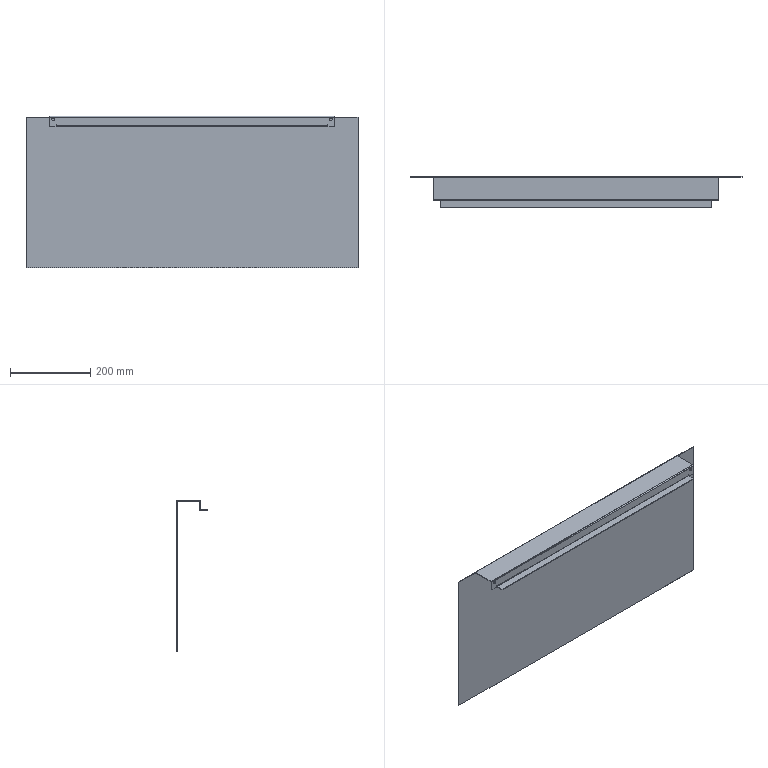Part | STEP file | Electrical Cabinet 2 | 1 solid | 40 faces | box 828 x 78 x 378 mm | volume 762303 mm3 | plane 24 | cylinder 16 | commonest cylinder face diameters 1 x9 7 x4 5 x3
STEP:
#1=CARTESIAN_POINT('',(684.62,-58.,322.807));
#2=VERTEX_POINT('',#1);
#3=CARTESIAN_POINT('',(684.62,-58.,329.807));
#4=VERTEX_POINT('',#3);
#5=CARTESIAN_POINT('',(684.62,-58.,326.307));
#6=DIRECTION('',(0.,1.,0.));
#7=DIRECTION('',(0.,0.,-1.));
#8=AXIS2_PLACEMENT_3D('',#5,#6,#7);
#9=CIRCLE('',#8,3.5);
#10=EDGE_CURVE('',#2,#4,#9,.T.);
#11=ORIENTED_EDGE('',*,*,#10,.T.);
#12=CARTESIAN_POINT('',(684.62,-60.,329.807));
#13=VERTEX_POINT('',#12);
#14=CARTESIAN_POINT('',(684.62,-50.,329.807));
#15=DIRECTION('',(0.,-1.,0.));
#16=VECTOR('',#15,1000.);
#17=LINE('',#14,#16);
#18=EDGE_CURVE('',#4,#13,#17,.T.);
#19=ORIENTED_EDGE('',*,*,#18,.T.);
#20=CARTESIAN_POINT('',(684.62,-60.,322.807));
#21=VERTEX_POINT('',#20);
#22=CARTESIAN_POINT('',(684.62,-60.,326.307));
#23=DIRECTION('',(0.,1.,0.));
#24=DIRECTION('',(0.,0.,-1.));
#25=AXIS2_PLACEMENT_3D('',#22,#23,#24);
#26=CIRCLE('',#25,3.5);
#27=EDGE_CURVE('',#21,#13,#26,.T.);
#28=ORIENTED_EDGE('',*,*,#27,.F.);
#29=CARTESIAN_POINT('',(684.62,-50.,322.807));
#30=DIRECTION('',(0.,-1.,0.));
#31=VECTOR('',#30,1000.);
#32=LINE('',#29,#31);
#33=EDGE_CURVE('',#2,#21,#32,.T.);
#34=ORIENTED_EDGE('',*,*,#33,.F.);
#35=EDGE_LOOP('',(#11,#19,#28,#34));
#36=FACE_OUTER_BOUND('',#35,.T.);
#37=CARTESIAN_POINT('',(684.62,-50.,326.307));
#38=DIRECTION('',(0.,-1.,0.));
#39=DIRECTION('',(0.,0.,-1.));
#40=AXIS2_PLACEMENT_3D('',#37,#38,#39);
#41=CYLINDRICAL_SURFACE('',#40,3.5);
#42=ADVANCED_FACE('',(#36),#41,.F.);
#43=CARTESIAN_POINT('',(-7.38,-58.,322.807));
#44=VERTEX_POINT('',#43);
#45=CARTESIAN_POINT('',(-7.38,-58.,329.807));
#46=VERTEX_POINT('',#45);
#47=CARTESIAN_POINT('',(-7.38,-58.,326.307));
#48=DIRECTION('',(0.,1.,0.));
#49=DIRECTION('',(0.,0.,-1.));
#50=AXIS2_PLACEMENT_3D('',#47,#48,#49);
#51=CIRCLE('',#50,3.5);
#52=EDGE_CURVE('',#44,#46,#51,.T.);
#53=ORIENTED_EDGE('',*,*,#52,.T.);
#54=CARTESIAN_POINT('',(-7.38,-60.,329.807));
#55=VERTEX_POINT('',#54);
#56=CARTESIAN_POINT('',(-7.38,-50.,329.807));
#57=DIRECTION('',(0.,-1.,0.));
#58=VECTOR('',#57,1000.);
#59=LINE('',#56,#58);
#60=EDGE_CURVE('',#46,#55,#59,.T.);
#61=ORIENTED_EDGE('',*,*,#60,.T.);
#62=CARTESIAN_POINT('',(-7.38,-60.,322.807));
#63=VERTEX_POINT('',#62);
#64=CARTESIAN_POINT('',(-7.38,-60.,326.307));
#65=DIRECTION('',(0.,1.,0.));
#66=DIRECTION('',(0.,0.,-1.));
#67=AXIS2_PLACEMENT_3D('',#64,#65,#66);
#68=CIRCLE('',#67,3.5);
#69=EDGE_CURVE('',#63,#55,#68,.T.);
#70=ORIENTED_EDGE('',*,*,#69,.F.);
#71=CARTESIAN_POINT('',(-7.38,-50.,322.807));
#72=DIRECTION('',(0.,-1.,0.));
#73=VECTOR('',#72,1000.);
#74=LINE('',#71,#73);
#75=EDGE_CURVE('',#44,#63,#74,.T.);
#76=ORIENTED_EDGE('',*,*,#75,.F.);
#77=EDGE_LOOP('',(#53,#61,#70,#76));
#78=FACE_OUTER_BOUND('',#77,.T.);
#79=CARTESIAN_POINT('',(-7.38,-50.,326.307));
#80=DIRECTION('',(0.,-1.,0.));
#81=DIRECTION('',(0.,0.,-1.));
#82=AXIS2_PLACEMENT_3D('',#79,#80,#81);
#83=CYLINDRICAL_SURFACE('',#82,3.5);
#84=ADVANCED_FACE('',(#78),#83,.F.);
#85=CARTESIAN_POINT('',(677.12,-60.,313.307));
#86=VERTEX_POINT('',#85);
#87=CARTESIAN_POINT('',(677.62,-60.,312.807));
#88=VERTEX_POINT('',#87);
#89=CARTESIAN_POINT('',(677.12,-60.,312.807));
#90=DIRECTION('',(0.,1.,0.));
#91=DIRECTION('',(0.,0.,1.));
#92=AXIS2_PLACEMENT_3D('',#89,#90,#91);
#93=CIRCLE('',#92,0.5);
#94=EDGE_CURVE('',#86,#88,#93,.T.);
#95=ORIENTED_EDGE('',*,*,#94,.F.);
#96=CARTESIAN_POINT('',(677.12,-58.,313.307));
#97=VERTEX_POINT('',#96);
#98=CARTESIAN_POINT('',(677.12,-60.,313.307));
#99=DIRECTION('',(0.,1.,0.));
#100=VECTOR('',#99,1000.);
#101=LINE('',#98,#100);
#102=EDGE_CURVE('',#86,#97,#101,.T.);
#103=ORIENTED_EDGE('',*,*,#102,.T.);
#104=CARTESIAN_POINT('',(677.62,-58.,312.807));
#105=VERTEX_POINT('',#104);
#106=CARTESIAN_POINT('',(677.12,-58.,312.807));
#107=DIRECTION('',(0.,-1.,0.));
#108=DIRECTION('',(0.,0.,1.));
#109=AXIS2_PLACEMENT_3D('',#106,#107,#108);
#110=CIRCLE('',#109,0.5);
#111=EDGE_CURVE('',#105,#97,#110,.T.);
#112=ORIENTED_EDGE('',*,*,#111,.F.);
#113=CARTESIAN_POINT('',(677.62,-60.,312.807));
#114=DIRECTION('',(0.,1.,0.));
#115=VECTOR('',#114,1000.);
#116=LINE('',#113,#115);
#117=EDGE_CURVE('',#88,#105,#116,.T.);
#118=ORIENTED_EDGE('',*,*,#117,.F.);
#119=EDGE_LOOP('',(#95,#103,#112,#118));
#120=FACE_OUTER_BOUND('',#119,.T.);
#121=CARTESIAN_POINT('',(677.12,-60.,312.807));
#122=DIRECTION('',(0.,1.,0.));
#123=DIRECTION('',(0.,0.,1.));
#124=AXIS2_PLACEMENT_3D('',#121,#122,#123);
#125=CYLINDRICAL_SURFACE('',#124,0.5);
#126=ADVANCED_FACE('',(#120),#125,.F.);
#127=CARTESIAN_POINT('',(0.1199,-60.,313.307));
#128=VERTEX_POINT('',#127);
#129=CARTESIAN_POINT('',(0.6199,-60.,312.807));
#130=VERTEX_POINT('',#129);
#131=CARTESIAN_POINT('',(0.1199,-60.,312.807));
#132=DIRECTION('',(0.,1.,0.));
#133=DIRECTION('',(0.,0.,1.));
#134=AXIS2_PLACEMENT_3D('',#131,#132,#133);
#135=CIRCLE('',#134,0.5);
#136=EDGE_CURVE('',#128,#130,#135,.T.);
#137=ORIENTED_EDGE('',*,*,#136,.F.);
#138=CARTESIAN_POINT('',(0.1199,-58.,313.307));
#139=VERTEX_POINT('',#138);
#140=CARTESIAN_POINT('',(0.1199,-60.,313.307));
#141=DIRECTION('',(0.,1.,0.));
#142=VECTOR('',#141,1000.);
#143=LINE('',#140,#142);
#144=EDGE_CURVE('',#128,#139,#143,.T.);
#145=ORIENTED_EDGE('',*,*,#144,.T.);
#146=CARTESIAN_POINT('',(0.6199,-58.,312.807));
#147=VERTEX_POINT('',#146);
#148=CARTESIAN_POINT('',(0.1199,-58.,312.807));
#149=DIRECTION('',(0.,-1.,0.));
#150=DIRECTION('',(0.,0.,1.));
#151=AXIS2_PLACEMENT_3D('',#148,#149,#150);
#152=CIRCLE('',#151,0.5);
#153=EDGE_CURVE('',#147,#139,#152,.T.);
#154=ORIENTED_EDGE('',*,*,#153,.F.);
#155=CARTESIAN_POINT('',(0.6199,-60.,312.807));
#156=DIRECTION('',(0.,1.,0.));
#157=VECTOR('',#156,1000.);
#158=LINE('',#155,#157);
#159=EDGE_CURVE('',#130,#147,#158,.T.);
#160=ORIENTED_EDGE('',*,*,#159,.F.);
#161=EDGE_LOOP('',(#137,#145,#154,#160));
#162=FACE_OUTER_BOUND('',#161,.T.);
#163=CARTESIAN_POINT('',(0.1199,-60.,312.807));
#164=DIRECTION('',(0.,1.,0.));
#165=DIRECTION('',(0.,0.,1.));
#166=AXIS2_PLACEMENT_3D('',#163,#164,#165);
#167=CYLINDRICAL_SURFACE('',#166,0.5);
#168=ADVANCED_FACE('',(#162),#167,.F.);
#169=CARTESIAN_POINT('',(695.62,-2.,332.307));
#170=VERTEX_POINT('',#169);
#171=CARTESIAN_POINT('',(752.62,-2.,332.307));
#172=VERTEX_POINT('',#171);
#173=CARTESIAN_POINT('',(0.,-2.,332.307));
#174=DIRECTION('',(1.,0.,0.));
#175=VECTOR('',#174,1000.);
#176=LINE('',#173,#175);
#177=EDGE_CURVE('',#170,#172,#176,.T.);
#178=ORIENTED_EDGE('',*,*,#177,.F.);
#179=CARTESIAN_POINT('',(695.62,-2.,330.807));
#180=VERTEX_POINT('',#179);
#181=CARTESIAN_POINT('',(695.62,-2.,330.807));
#182=DIRECTION('',(0.,0.,1.));
#183=VECTOR('',#182,1000.);
#184=LINE('',#181,#183);
#185=EDGE_CURVE('',#180,#170,#184,.T.);
#186=ORIENTED_EDGE('',*,*,#185,.F.);
#187=CARTESIAN_POINT('',(694.62,-2.,330.807));
#188=VERTEX_POINT('',#187);
#189=CARTESIAN_POINT('',(695.12,-2.,330.807));
#190=DIRECTION('',(0.,1.,0.));
#191=DIRECTION('',(0.,0.,1.));
#192=AXIS2_PLACEMENT_3D('',#189,#190,#191);
#193=CIRCLE('',#192,0.5);
#194=EDGE_CURVE('',#180,#188,#193,.T.);
#195=ORIENTED_EDGE('',*,*,#194,.T.);
#196=CARTESIAN_POINT('',(694.62,-2.,331.807));
#197=VERTEX_POINT('',#196);
#198=CARTESIAN_POINT('',(694.62,-2.,331.807));
#199=DIRECTION('',(0.,0.,-1.));
#200=VECTOR('',#199,1000.);
#201=LINE('',#198,#200);
#202=EDGE_CURVE('',#197,#188,#201,.T.);
#203=ORIENTED_EDGE('',*,*,#202,.F.);
#204=CARTESIAN_POINT('',(-17.38,-2.,331.807));
#205=VERTEX_POINT('',#204);
#206=CARTESIAN_POINT('',(0.,-2.,331.807));
#207=DIRECTION('',(1.,0.,0.));
#208=VECTOR('',#207,1000.);
#209=LINE('',#206,#208);
#210=EDGE_CURVE('',#205,#197,#209,.T.);
#211=ORIENTED_EDGE('',*,*,#210,.F.);
#212=CARTESIAN_POINT('',(-17.38,-2.,330.807));
#213=VERTEX_POINT('',#212);
#214=CARTESIAN_POINT('',(-17.38,-2.,330.807));
#215=DIRECTION('',(0.,0.,1.));
#216=VECTOR('',#215,1000.);
#217=LINE('',#214,#216);
#218=EDGE_CURVE('',#213,#205,#217,.T.);
#219=ORIENTED_EDGE('',*,*,#218,.F.);
#220=CARTESIAN_POINT('',(-18.38,-2.,330.807));
#221=VERTEX_POINT('',#220);
#222=CARTESIAN_POINT('',(-17.88,-2.,330.807));
#223=DIRECTION('',(0.,1.,0.));
#224=DIRECTION('',(0.,0.,1.));
#225=AXIS2_PLACEMENT_3D('',#222,#223,#224);
#226=CIRCLE('',#225,0.5);
#227=EDGE_CURVE('',#213,#221,#226,.T.);
#228=ORIENTED_EDGE('',*,*,#227,.T.);
#229=CARTESIAN_POINT('',(-18.38,-2.,332.307));
#230=VERTEX_POINT('',#229);
#231=CARTESIAN_POINT('',(-18.38,-2.,334.307));
#232=DIRECTION('',(0.,0.,-1.));
#233=VECTOR('',#232,1000.);
#234=LINE('',#231,#233);
#235=EDGE_CURVE('',#230,#221,#234,.T.);
#236=ORIENTED_EDGE('',*,*,#235,.F.);
#237=CARTESIAN_POINT('',(-75.38,-2.,332.307));
#238=VERTEX_POINT('',#237);
#239=CARTESIAN_POINT('',(0.,-2.,332.307));
#240=DIRECTION('',(1.,0.,0.));
#241=VECTOR('',#240,1000.);
#242=LINE('',#239,#241);
#243=EDGE_CURVE('',#238,#230,#242,.T.);
#244=ORIENTED_EDGE('',*,*,#243,.F.);
#245=CARTESIAN_POINT('',(-75.38,-2.,-43.693));
#246=VERTEX_POINT('',#245);
#247=CARTESIAN_POINT('',(-75.38,-2.,0.));
#248=DIRECTION('',(0.,0.,1.));
#249=VECTOR('',#248,1000.);
#250=LINE('',#247,#249);
#251=EDGE_CURVE('',#246,#238,#250,.T.);
#252=ORIENTED_EDGE('',*,*,#251,.F.);
#253=CARTESIAN_POINT('',(752.62,-2.,-43.693));
#254=VERTEX_POINT('',#253);
#255=CARTESIAN_POINT('',(0.,-2.,-43.693));
#256=DIRECTION('',(-1.,0.,0.));
#257=VECTOR('',#256,1000.);
#258=LINE('',#255,#257);
#259=EDGE_CURVE('',#254,#246,#258,.T.);
#260=ORIENTED_EDGE('',*,*,#259,.F.);
#261=CARTESIAN_POINT('',(752.62,-2.,0.));
#262=DIRECTION('',(0.,0.,-1.));
#263=VECTOR('',#262,1000.);
#264=LINE('',#261,#263);
#265=EDGE_CURVE('',#172,#254,#264,.T.);
#266=ORIENTED_EDGE('',*,*,#265,.F.);
#267=EDGE_LOOP('',(#178,#186,#195,#203,#211,#219,#228,#236,#244,#252,#260,#266));
#268=FACE_OUTER_BOUND('',#267,.T.);
#269=CARTESIAN_POINT('',(0.,-2.,0.));
#270=DIRECTION('',(0.,1.,0.));
#271=DIRECTION('',(0.,0.,1.));
#272=AXIS2_PLACEMENT_3D('',#269,#270,#271);
#273=PLANE('',#272);
#274=ADVANCED_FACE('',(#268),#273,.F.);
#275=CARTESIAN_POINT('',(752.62,0.,-43.693));
#276=VERTEX_POINT('',#275);
#277=CARTESIAN_POINT('',(752.62,-2.,-43.693));
#278=DIRECTION('',(0.,1.,0.));
#279=VECTOR('',#278,1000.);
#280=LINE('',#277,#279);
#281=EDGE_CURVE('',#254,#276,#280,.T.);
#282=ORIENTED_EDGE('',*,*,#281,.T.);
#283=CARTESIAN_POINT('',(752.62,0.,332.307));
#284=VERTEX_POINT('',#283);
#285=CARTESIAN_POINT('',(752.62,0.,-43.693));
#286=DIRECTION('',(0.,0.,1.));
#287=VECTOR('',#286,1000.);
#288=LINE('',#285,#287);
#289=EDGE_CURVE('',#276,#284,#288,.T.);
#290=ORIENTED_EDGE('',*,*,#289,.T.);
#291=CARTESIAN_POINT('',(752.62,-2.,332.307));
#292=DIRECTION('',(0.,-1.,0.));
#293=VECTOR('',#292,1000.);
#294=LINE('',#291,#293);
#295=EDGE_CURVE('',#284,#172,#294,.T.);
#296=ORIENTED_EDGE('',*,*,#295,.T.);
#297=ORIENTED_EDGE('',*,*,#265,.T.);
#298=EDGE_LOOP('',(#282,#290,#296,#297));
#299=FACE_OUTER_BOUND('',#298,.T.);
#300=CARTESIAN_POINT('',(752.62,-2.,-43.693));
#301=DIRECTION('',(1.,0.,0.));
#302=DIRECTION('',(0.,0.,-1.));
#303=AXIS2_PLACEMENT_3D('',#300,#301,#302);
#304=PLANE('',#303);
#305=ADVANCED_FACE('',(#299),#304,.T.);
#306=CARTESIAN_POINT('',(695.62,0.,332.307));
#307=VERTEX_POINT('',#306);
#308=CARTESIAN_POINT('',(695.62,0.,332.307));
#309=DIRECTION('',(1.,0.,0.));
#310=VECTOR('',#309,1000.);
#311=LINE('',#308,#310);
#312=EDGE_CURVE('',#307,#284,#311,.T.);
#313=ORIENTED_EDGE('',*,*,#312,.F.);
#314=CARTESIAN_POINT('',(695.62,-10.,332.307));
#315=DIRECTION('',(0.,1.,0.));
#316=VECTOR('',#315,1000.);
#317=LINE('',#314,#316);
#318=EDGE_CURVE('',#170,#307,#317,.T.);
#319=ORIENTED_EDGE('',*,*,#318,.F.);
#320=ORIENTED_EDGE('',*,*,#177,.T.);
#321=ORIENTED_EDGE('',*,*,#295,.F.);
#322=EDGE_LOOP('',(#313,#319,#320,#321));
#323=FACE_OUTER_BOUND('',#322,.T.);
#324=CARTESIAN_POINT('',(695.62,-10.,332.307));
#325=DIRECTION('',(0.,0.,-1.));
#326=DIRECTION('',(-1.,0.,0.));
#327=AXIS2_PLACEMENT_3D('',#324,#325,#326);
#328=PLANE('',#327);
#329=ADVANCED_FACE('',(#323),#328,.F.);
#330=CARTESIAN_POINT('',(694.62,-2.5,332.307));
#331=VERTEX_POINT('',#330);
#332=CARTESIAN_POINT('',(694.62,-2.5,331.807));
#333=DIRECTION('',(-1.,0.,0.));
#334=DIRECTION('',(0.,0.,1.));
#335=AXIS2_PLACEMENT_3D('',#332,#333,#334);
#336=CIRCLE('',#335,0.5);
#337=EDGE_CURVE('',#331,#197,#336,.T.);
#338=ORIENTED_EDGE('',*,*,#337,.F.);
#339=CARTESIAN_POINT('',(-17.38,-2.5,332.307));
#340=VERTEX_POINT('',#339);
#341=CARTESIAN_POINT('',(-17.38,-2.5,332.307));
#342=DIRECTION('',(1.,0.,0.));
#343=VECTOR('',#342,1000.);
#344=LINE('',#341,#343);
#345=EDGE_CURVE('',#340,#331,#344,.T.);
#346=ORIENTED_EDGE('',*,*,#345,.F.);
#347=CARTESIAN_POINT('',(-17.38,-2.5,331.807));
#348=DIRECTION('',(-1.,0.,0.));
#349=DIRECTION('',(0.,0.,1.));
#350=AXIS2_PLACEMENT_3D('',#347,#348,#349);
#351=CIRCLE('',#350,0.5);
#352=EDGE_CURVE('',#340,#205,#351,.T.);
#353=ORIENTED_EDGE('',*,*,#352,.T.);
#354=ORIENTED_EDGE('',*,*,#210,.T.);
#355=EDGE_LOOP('',(#338,#346,#353,#354));
#356=FACE_OUTER_BOUND('',#355,.T.);
#357=CARTESIAN_POINT('',(-17.38,-2.5,331.807));
#358=DIRECTION('',(-1.,0.,0.));
#359=DIRECTION('',(0.,0.,1.));
#360=AXIS2_PLACEMENT_3D('',#357,#358,#359);
#361=CYLINDRICAL_SURFACE('',#360,0.5);
#362=ADVANCED_FACE('',(#356),#361,.F.);
#363=CARTESIAN_POINT('',(-75.38,0.,332.307));
#364=VERTEX_POINT('',#363);
#365=CARTESIAN_POINT('',(-18.38,0.,332.307));
#366=VERTEX_POINT('',#365);
#367=CARTESIAN_POINT('',(-75.38,0.,332.307));
#368=DIRECTION('',(1.,0.,0.));
#369=VECTOR('',#368,1000.);
#370=LINE('',#367,#369);
#371=EDGE_CURVE('',#364,#366,#370,.T.);
#372=ORIENTED_EDGE('',*,*,#371,.F.);
#373=CARTESIAN_POINT('',(-75.38,-10.,332.307));
#374=DIRECTION('',(0.,1.,0.));
#375=VECTOR('',#374,1000.);
#376=LINE('',#373,#375);
#377=EDGE_CURVE('',#238,#364,#376,.T.);
#378=ORIENTED_EDGE('',*,*,#377,.F.);
#379=ORIENTED_EDGE('',*,*,#243,.T.);
#380=CARTESIAN_POINT('',(-18.38,-10.,332.307));
#381=DIRECTION('',(0.,-1.,0.));
#382=VECTOR('',#381,1000.);
#383=LINE('',#380,#382);
#384=EDGE_CURVE('',#366,#230,#383,.T.);
#385=ORIENTED_EDGE('',*,*,#384,.F.);
#386=EDGE_LOOP('',(#372,#378,#379,#385));
#387=FACE_OUTER_BOUND('',#386,.T.);
#388=CARTESIAN_POINT('',(-75.38,-10.,332.307));
#389=DIRECTION('',(0.,0.,-1.));
#390=DIRECTION('',(-1.,0.,0.));
#391=AXIS2_PLACEMENT_3D('',#388,#389,#390);
#392=PLANE('',#391);
#393=ADVANCED_FACE('',(#387),#392,.F.);
#394=CARTESIAN_POINT('',(-75.38,0.,-43.693));
#395=VERTEX_POINT('',#394);
#396=CARTESIAN_POINT('',(-75.38,-2.,-43.693));
#397=DIRECTION('',(0.,-1.,0.));
#398=VECTOR('',#397,1000.);
#399=LINE('',#396,#398);
#400=EDGE_CURVE('',#395,#246,#399,.T.);
#401=ORIENTED_EDGE('',*,*,#400,.T.);
#402=ORIENTED_EDGE('',*,*,#251,.T.);
#403=ORIENTED_EDGE('',*,*,#377,.T.);
#404=CARTESIAN_POINT('',(-75.38,0.,-43.693));
#405=DIRECTION('',(0.,0.,-1.));
#406=VECTOR('',#405,1000.);
#407=LINE('',#404,#406);
#408=EDGE_CURVE('',#364,#395,#407,.T.);
#409=ORIENTED_EDGE('',*,*,#408,.T.);
#410=EDGE_LOOP('',(#401,#402,#403,#409));
#411=FACE_OUTER_BOUND('',#410,.T.);
#412=CARTESIAN_POINT('',(-75.38,-2.,-43.693));
#413=DIRECTION('',(-1.,0.,0.));
#414=DIRECTION('',(0.,0.,1.));
#415=AXIS2_PLACEMENT_3D('',#412,#413,#414);
#416=PLANE('',#415);
#417=ADVANCED_FACE('',(#411),#416,.T.);
#418=ORIENTED_EDGE('',*,*,#259,.T.);
#419=ORIENTED_EDGE('',*,*,#400,.F.);
#420=CARTESIAN_POINT('',(-75.38,0.,-43.693));
#421=DIRECTION('',(1.,0.,0.));
#422=VECTOR('',#421,1000.);
#423=LINE('',#420,#422);
#424=EDGE_CURVE('',#395,#276,#423,.T.);
#425=ORIENTED_EDGE('',*,*,#424,.T.);
#426=ORIENTED_EDGE('',*,*,#281,.F.);
#427=EDGE_LOOP('',(#418,#419,#425,#426));
#428=FACE_OUTER_BOUND('',#427,.T.);
#429=CARTESIAN_POINT('',(-75.38,-2.,-43.693));
#430=DIRECTION('',(0.,0.,-1.));
#431=DIRECTION('',(-1.,0.,0.));
#432=AXIS2_PLACEMENT_3D('',#429,#430,#431);
#433=PLANE('',#432);
#434=ADVANCED_FACE('',(#428),#433,.T.);
#435=CARTESIAN_POINT('',(694.62,0.,330.807));
#436=VERTEX_POINT('',#435);
#437=CARTESIAN_POINT('',(695.62,0.,330.807));
#438=VERTEX_POINT('',#437);
#439=CARTESIAN_POINT('',(695.12,0.,330.807));
#440=DIRECTION('',(0.,-1.,0.));
#441=DIRECTION('',(0.,0.,1.));
#442=AXIS2_PLACEMENT_3D('',#439,#440,#441);
#443=CIRCLE('',#442,0.5);
#444=EDGE_CURVE('',#436,#438,#443,.T.);
#445=ORIENTED_EDGE('',*,*,#444,.T.);
#446=CARTESIAN_POINT('',(695.62,0.,0.));
#447=DIRECTION('',(0.,0.,1.));
#448=VECTOR('',#447,1000.);
#449=LINE('',#446,#448);
#450=EDGE_CURVE('',#438,#307,#449,.T.);
#451=ORIENTED_EDGE('',*,*,#450,.T.);
#452=ORIENTED_EDGE('',*,*,#312,.T.);
#453=ORIENTED_EDGE('',*,*,#289,.F.);
#454=ORIENTED_EDGE('',*,*,#424,.F.);
#455=ORIENTED_EDGE('',*,*,#408,.F.);
#456=ORIENTED_EDGE('',*,*,#371,.T.);
#457=CARTESIAN_POINT('',(-18.38,0.,330.807));
#458=VERTEX_POINT('',#457);
#459=CARTESIAN_POINT('',(-18.38,0.,0.));
#460=DIRECTION('',(0.,0.,-1.));
#461=VECTOR('',#460,1000.);
#462=LINE('',#459,#461);
#463=EDGE_CURVE('',#366,#458,#462,.T.);
#464=ORIENTED_EDGE('',*,*,#463,.T.);
#465=CARTESIAN_POINT('',(-17.38,0.,330.807));
#466=VERTEX_POINT('',#465);
#467=CARTESIAN_POINT('',(-17.88,0.,330.807));
#468=DIRECTION('',(0.,-1.,0.));
#469=DIRECTION('',(0.,0.,1.));
#470=AXIS2_PLACEMENT_3D('',#467,#468,#469);
#471=CIRCLE('',#470,0.5);
#472=EDGE_CURVE('',#458,#466,#471,.T.);
#473=ORIENTED_EDGE('',*,*,#472,.T.);
#474=CARTESIAN_POINT('',(-17.38,0.,331.807));
#475=VERTEX_POINT('',#474);
#476=CARTESIAN_POINT('',(-17.38,0.,330.807));
#477=DIRECTION('',(0.,0.,-1.));
#478=VECTOR('',#477,1000.);
#479=LINE('',#476,#478);
#480=EDGE_CURVE('',#475,#466,#479,.T.);
#481=ORIENTED_EDGE('',*,*,#480,.F.);
#482=CARTESIAN_POINT('',(694.62,0.,331.807));
#483=VERTEX_POINT('',#482);
#484=CARTESIAN_POINT('',(0.,0.,331.807));
#485=DIRECTION('',(1.,0.,0.));
#486=VECTOR('',#485,1000.);
#487=LINE('',#484,#486);
#488=EDGE_CURVE('',#475,#483,#487,.T.);
#489=ORIENTED_EDGE('',*,*,#488,.T.);
#490=CARTESIAN_POINT('',(694.62,0.,331.807));
#491=DIRECTION('',(0.,0.,1.));
#492=VECTOR('',#491,1000.);
#493=LINE('',#490,#492);
#494=EDGE_CURVE('',#436,#483,#493,.T.);
#495=ORIENTED_EDGE('',*,*,#494,.F.);
#496=EDGE_LOOP('',(#445,#451,#452,#453,#454,#455,#456,#464,#473,#481,#489,#495));
#497=FACE_OUTER_BOUND('',#496,.T.);
#498=CARTESIAN_POINT('',(0.,0.,0.));
#499=DIRECTION('',(0.,1.,0.));
#500=DIRECTION('',(0.,0.,1.));
#501=AXIS2_PLACEMENT_3D('',#498,#499,#500);
#502=PLANE('',#501);
#503=ADVANCED_FACE('',(#497),#502,.T.);
#504=CARTESIAN_POINT('',(695.62,-2.,330.807));
#505=DIRECTION('',(0.,-1.,0.));
#506=VECTOR('',#505,1000.);
#507=LINE('',#504,#506);
#508=EDGE_CURVE('',#438,#180,#507,.T.);
#509=ORIENTED_EDGE('',*,*,#508,.T.);
#510=ORIENTED_EDGE('',*,*,#185,.T.);
#511=ORIENTED_EDGE('',*,*,#318,.T.);
#512=ORIENTED_EDGE('',*,*,#450,.F.);
#513=EDGE_LOOP('',(#509,#510,#511,#512));
#514=FACE_OUTER_BOUND('',#513,.T.);
#515=CARTESIAN_POINT('',(695.62,-2.,330.807));
#516=DIRECTION('',(-1.,0.,0.));
#517=DIRECTION('',(0.,0.,1.));
#518=AXIS2_PLACEMENT_3D('',#515,#516,#517);
#519=PLANE('',#518);
#520=ADVANCED_FACE('',(#514),#519,.T.);
#521=CARTESIAN_POINT('',(-17.38,-57.5,332.307));
#522=VERTEX_POINT('',#521);
#523=CARTESIAN_POINT('',(-17.38,0.,332.307));
#524=DIRECTION('',(0.,-1.,0.));
#525=VECTOR('',#524,1000.);
#526=LINE('',#523,#525);
#527=EDGE_CURVE('',#340,#522,#526,.T.);
#528=ORIENTED_EDGE('',*,*,#527,.F.);
#529=ORIENTED_EDGE('',*,*,#345,.T.);
#530=CARTESIAN_POINT('',(694.62,-57.5,332.307));
#531=VERTEX_POINT('',#530);
#532=CARTESIAN_POINT('',(694.62,0.,332.307));
#533=DIRECTION('',(0.,1.,0.));
#534=VECTOR('',#533,1000.);
#535=LINE('',#532,#534);
#536=EDGE_CURVE('',#531,#331,#535,.T.);
#537=ORIENTED_EDGE('',*,*,#536,.F.);
#538=CARTESIAN_POINT('',(0.,-57.5,332.307));
#539=DIRECTION('',(1.,0.,0.));
#540=VECTOR('',#539,1000.);
#541=LINE('',#538,#540);
#542=EDGE_CURVE('',#522,#531,#541,.T.);
#543=ORIENTED_EDGE('',*,*,#542,.F.);
#544=EDGE_LOOP('',(#528,#529,#537,#543));
#545=FACE_OUTER_BOUND('',#544,.T.);
#546=CARTESIAN_POINT('',(0.,0.,332.307));
#547=DIRECTION('',(0.,0.,1.));
#548=DIRECTION('',(0.,-1.,0.));
#549=AXIS2_PLACEMENT_3D('',#546,#547,#548);
#550=PLANE('',#549);
#551=ADVANCED_FACE('',(#545),#550,.F.);
#552=CARTESIAN_POINT('',(-18.38,-2.,330.807));
#553=DIRECTION('',(0.,1.,0.));
#554=VECTOR('',#553,1000.);
#555=LINE('',#552,#554);
#556=EDGE_CURVE('',#221,#458,#555,.T.);
#557=ORIENTED_EDGE('',*,*,#556,.T.);
#558=ORIENTED_EDGE('',*,*,#463,.F.);
#559=ORIENTED_EDGE('',*,*,#384,.T.);
#560=ORIENTED_EDGE('',*,*,#235,.T.);
#561=EDGE_LOOP('',(#557,#558,#559,#560));
#562=FACE_OUTER_BOUND('',#561,.T.);
#563=CARTESIAN_POINT('',(-18.38,-2.,334.307));
#564=DIRECTION('',(1.,0.,0.));
#565=DIRECTION('',(0.,0.,-1.));
#566=AXIS2_PLACEMENT_3D('',#563,#564,#565);
#567=PLANE('',#566);
#568=ADVANCED_FACE('',(#562),#567,.T.);
#569=CARTESIAN_POINT('',(-17.38,-2.5,334.307));
#570=VERTEX_POINT('',#569);
#571=CARTESIAN_POINT('',(694.62,-2.5,334.307));
#572=VERTEX_POINT('',#571);
#573=CARTESIAN_POINT('',(-17.38,-2.5,334.307));
#574=DIRECTION('',(1.,0.,0.));
#575=VECTOR('',#574,1000.);
#576=LINE('',#573,#575);
#577=EDGE_CURVE('',#570,#572,#576,.T.);
#578=ORIENTED_EDGE('',*,*,#577,.T.);
#579=CARTESIAN_POINT('',(694.62,-2.5,331.807));
#580=DIRECTION('',(-1.,0.,0.));
#581=DIRECTION('',(0.,0.,1.));
#582=AXIS2_PLACEMENT_3D('',#579,#580,#581);
#583=CIRCLE('',#582,2.5);
#584=EDGE_CURVE('',#572,#483,#583,.T.);
#585=ORIENTED_EDGE('',*,*,#584,.T.);
#586=ORIENTED_EDGE('',*,*,#488,.F.);
#587=CARTESIAN_POINT('',(-17.38,-2.5,331.807));
#588=DIRECTION('',(1.,0.,0.));
#589=DIRECTION('',(0.,0.,1.));
#590=AXIS2_PLACEMENT_3D('',#587,#588,#589);
#591=CIRCLE('',#590,2.5);
#592=EDGE_CURVE('',#475,#570,#591,.T.);
#593=ORIENTED_EDGE('',*,*,#592,.T.);
#594=EDGE_LOOP('',(#578,#585,#586,#593));
#595=FACE_OUTER_BOUND('',#594,.T.);
#596=CARTESIAN_POINT('',(-17.38,-2.5,331.807));
#597=DIRECTION('',(-1.,0.,0.));
#598=DIRECTION('',(0.,0.,1.));
#599=AXIS2_PLACEMENT_3D('',#596,#597,#598);
#600=CYLINDRICAL_SURFACE('',#599,2.5);
#601=ADVANCED_FACE('',(#595),#600,.T.);
#602=CARTESIAN_POINT('',(694.62,-2.,330.807));
#603=DIRECTION('',(0.,1.,0.));
#604=VECTOR('',#603,1000.);
#605=LINE('',#602,#604);
#606=EDGE_CURVE('',#188,#436,#605,.T.);
#607=ORIENTED_EDGE('',*,*,#606,.F.);
#608=ORIENTED_EDGE('',*,*,#194,.F.);
#609=ORIENTED_EDGE('',*,*,#508,.F.);
#610=ORIENTED_EDGE('',*,*,#444,.F.);
#611=EDGE_LOOP('',(#607,#608,#609,#610));
#612=FACE_OUTER_BOUND('',#611,.T.);
#613=CARTESIAN_POINT('',(695.12,-2.,330.807));
#614=DIRECTION('',(0.,1.,0.));
#615=DIRECTION('',(0.,0.,1.));
#616=AXIS2_PLACEMENT_3D('',#613,#614,#615);
#617=CYLINDRICAL_SURFACE('',#616,0.5);
#618=ADVANCED_FACE('',(#612),#617,.F.);
#619=CARTESIAN_POINT('',(694.62,-58.,331.807));
#620=VERTEX_POINT('',#619);
#621=CARTESIAN_POINT('',(694.62,-57.5,331.807));
#622=DIRECTION('',(-1.,0.,0.));
#623=DIRECTION('',(0.,0.,1.));
#624=AXIS2_PLACEMENT_3D('',#621,#622,#623);
#625=CIRCLE('',#624,0.5);
#626=EDGE_CURVE('',#620,#531,#625,.T.);
#627=ORIENTED_EDGE('',*,*,#626,.F.);
#628=CARTESIAN_POINT('',(-17.38,-58.,331.807));
#629=VERTEX_POINT('',#628);
#630=CARTESIAN_POINT('',(-17.38,-58.,331.807));
#631=DIRECTION('',(1.,0.,0.));
#632=VECTOR('',#631,1000.);
#633=LINE('',#630,#632);
#634=EDGE_CURVE('',#629,#620,#633,.T.);
#635=ORIENTED_EDGE('',*,*,#634,.F.);
#636=CARTESIAN_POINT('',(-17.38,-57.5,331.807));
#637=DIRECTION('',(-1.,0.,0.));
#638=DIRECTION('',(0.,0.,1.));
#639=AXIS2_PLACEMENT_3D('',#636,#637,#638);
#640=CIRCLE('',#639,0.5);
#641=EDGE_CURVE('',#629,#522,#640,.T.);
#642=ORIENTED_EDGE('',*,*,#641,.T.);
#643=ORIENTED_EDGE('',*,*,#542,.T.);
#644=EDGE_LOOP('',(#627,#635,#642,#643));
#645=FACE_OUTER_BOUND('',#644,.T.);
#646=CARTESIAN_POINT('',(-17.38,-57.5,331.807));
#647=DIRECTION('',(-1.,0.,0.));
#648=DIRECTION('',(0.,0.,1.));
#649=AXIS2_PLACEMENT_3D('',#646,#647,#648);
#650=CYLINDRICAL_SURFACE('',#649,0.5);
#651=ADVANCED_FACE('',(#645),#650,.F.);
#652=CARTESIAN_POINT('',(-17.38,-57.5,334.307));
#653=VERTEX_POINT('',#652);
#654=CARTESIAN_POINT('',(-17.38,-2.,334.307));
#655=DIRECTION('',(0.,1.,0.));
#656=VECTOR('',#655,1000.);
#657=LINE('',#654,#656);
#658=EDGE_CURVE('',#653,#570,#657,.T.);
#659=ORIENTED_EDGE('',*,*,#658,.T.);
#660=ORIENTED_EDGE('',*,*,#592,.F.);
#661=ORIENTED_EDGE('',*,*,#480,.T.);
#662=CARTESIAN_POINT('',(-17.38,-2.,330.807));
#663=DIRECTION('',(0.,-1.,0.));
#664=VECTOR('',#663,1000.);
#665=LINE('',#662,#664);
#666=EDGE_CURVE('',#466,#213,#665,.T.);
#667=ORIENTED_EDGE('',*,*,#666,.T.);
#668=ORIENTED_EDGE('',*,*,#218,.T.);
#669=ORIENTED_EDGE('',*,*,#352,.F.);
#670=ORIENTED_EDGE('',*,*,#527,.T.);
#671=ORIENTED_EDGE('',*,*,#641,.F.);
#672=CARTESIAN_POINT('',(-17.38,-58.,309.307));
#673=VERTEX_POINT('',#672);
#674=CARTESIAN_POINT('',(-17.38,-58.,0.));
#675=DIRECTION('',(0.,0.,-1.));
#676=VECTOR('',#675,1000.);
#677=LINE('',#674,#676);
#678=EDGE_CURVE('',#629,#673,#677,.T.);
#679=ORIENTED_EDGE('',*,*,#678,.T.);
#680=CARTESIAN_POINT('',(-17.38,-60.,309.307));
#681=VERTEX_POINT('',#680);
#682=CARTESIAN_POINT('',(-17.38,-60.,309.307));
#683=DIRECTION('',(0.,1.,0.));
#684=VECTOR('',#683,1000.);
#685=LINE('',#682,#684);
#686=EDGE_CURVE('',#681,#673,#685,.T.);
#687=ORIENTED_EDGE('',*,*,#686,.F.);
#688=CARTESIAN_POINT('',(-17.38,-60.,331.807));
#689=VERTEX_POINT('',#688);
#690=CARTESIAN_POINT('',(-17.38,-60.,332.307));
#691=DIRECTION('',(0.,0.,1.));
#692=VECTOR('',#691,1000.);
#693=LINE('',#690,#692);
#694=EDGE_CURVE('',#681,#689,#693,.T.);
#695=ORIENTED_EDGE('',*,*,#694,.T.);
#696=CARTESIAN_POINT('',(-17.38,-57.5,331.807));
#697=DIRECTION('',(1.,0.,0.));
#698=DIRECTION('',(0.,0.,1.));
#699=AXIS2_PLACEMENT_3D('',#696,#697,#698);
#700=CIRCLE('',#699,2.5);
#701=EDGE_CURVE('',#653,#689,#700,.T.);
#702=ORIENTED_EDGE('',*,*,#701,.F.);
#703=EDGE_LOOP('',(#659,#660,#661,#667,#668,#669,#670,#671,#679,#687,#695,#702));
#704=FACE_OUTER_BOUND('',#703,.T.);
#705=CARTESIAN_POINT('',(-17.38,-2.,334.307));
#706=DIRECTION('',(-1.,0.,0.));
#707=DIRECTION('',(0.,-1.,0.));
#708=AXIS2_PLACEMENT_3D('',#705,#706,#707);
#709=PLANE('',#708);
#710=ADVANCED_FACE('',(#704),#709,.T.);
#711=ORIENTED_EDGE('',*,*,#536,.T.);
#712=ORIENTED_EDGE('',*,*,#337,.T.);
#713=ORIENTED_EDGE('',*,*,#202,.T.);
#714=ORIENTED_EDGE('',*,*,#606,.T.);
#715=ORIENTED_EDGE('',*,*,#494,.T.);
#716=ORIENTED_EDGE('',*,*,#584,.F.);
#717=CARTESIAN_POINT('',(694.62,-57.5,334.307));
#718=VERTEX_POINT('',#717);
#719=CARTESIAN_POINT('',(694.62,-60.,334.307));
#720=DIRECTION('',(0.,-1.,0.));
#721=VECTOR('',#720,1000.);
#722=LINE('',#719,#721);
#723=EDGE_CURVE('',#572,#718,#722,.T.);
#724=ORIENTED_EDGE('',*,*,#723,.T.);
#725=CARTESIAN_POINT('',(694.62,-60.,331.807));
#726=VERTEX_POINT('',#725);
#727=CARTESIAN_POINT('',(694.62,-57.5,331.807));
#728=DIRECTION('',(1.,0.,0.));
#729=DIRECTION('',(0.,0.,1.));
#730=AXIS2_PLACEMENT_3D('',#727,#728,#729);
#731=CIRCLE('',#730,2.5);
#732=EDGE_CURVE('',#718,#726,#731,.T.);
#733=ORIENTED_EDGE('',*,*,#732,.T.);
#734=CARTESIAN_POINT('',(694.62,-60.,309.307));
#735=VERTEX_POINT('',#734);
#736=CARTESIAN_POINT('',(694.62,-60.,309.307));
#737=DIRECTION('',(0.,0.,-1.));
#738=VECTOR('',#737,1000.);
#739=LINE('',#736,#738);
#740=EDGE_CURVE('',#726,#735,#739,.T.);
#741=ORIENTED_EDGE('',*,*,#740,.T.);
#742=CARTESIAN_POINT('',(694.62,-58.,309.307));
#743=VERTEX_POINT('',#742);
#744=CARTESIAN_POINT('',(694.62,-60.,309.307));
#745=DIRECTION('',(0.,1.,0.));
#746=VECTOR('',#745,1000.);
#747=LINE('',#744,#746);
#748=EDGE_CURVE('',#735,#743,#747,.T.);
#749=ORIENTED_EDGE('',*,*,#748,.T.);
#750=CARTESIAN_POINT('',(694.62,-58.,0.));
#751=DIRECTION('',(0.,0.,1.));
#752=VECTOR('',#751,1000.);
#753=LINE('',#750,#752);
#754=EDGE_CURVE('',#743,#620,#753,.T.);
#755=ORIENTED_EDGE('',*,*,#754,.T.);
#756=ORIENTED_EDGE('',*,*,#626,.T.);
#757=EDGE_LOOP('',(#711,#712,#713,#714,#715,#716,#724,#733,#741,#749,#755,#756));
#758=FACE_OUTER_BOUND('',#757,.T.);
#759=CARTESIAN_POINT('',(694.62,-60.,334.307));
#760=DIRECTION('',(1.,0.,0.));
#761=DIRECTION('',(0.,0.,-1.));
#762=AXIS2_PLACEMENT_3D('',#759,#760,#761);
#763=PLANE('',#762);
#764=ADVANCED_FACE('',(#758),#763,.T.);
#765=ORIENTED_EDGE('',*,*,#556,.F.);
#766=ORIENTED_EDGE('',*,*,#227,.F.);
#767=ORIENTED_EDGE('',*,*,#666,.F.);
#768=ORIENTED_EDGE('',*,*,#472,.F.);
#769=EDGE_LOOP('',(#765,#766,#767,#768));
#770=FACE_OUTER_BOUND('',#769,.T.);
#771=CARTESIAN_POINT('',(-17.88,-2.,330.807));
#772=DIRECTION('',(0.,1.,0.));
#773=DIRECTION('',(0.,0.,1.));
#774=AXIS2_PLACEMENT_3D('',#771,#772,#773);
#775=CYLINDRICAL_SURFACE('',#774,0.5);
#776=ADVANCED_FACE('',(#770),#775,.F.);
#777=ORIENTED_EDGE('',*,*,#723,.F.);
#778=ORIENTED_EDGE('',*,*,#577,.F.);
#779=ORIENTED_EDGE('',*,*,#658,.F.);
#780=CARTESIAN_POINT('',(0.,-57.5,334.307));
#781=DIRECTION('',(1.,0.,0.));
#782=VECTOR('',#781,1000.);
#783=LINE('',#780,#782);
#784=EDGE_CURVE('',#653,#718,#783,.T.);
#785=ORIENTED_EDGE('',*,*,#784,.T.);
#786=EDGE_LOOP('',(#777,#778,#779,#785));
#787=FACE_OUTER_BOUND('',#786,.T.);
#788=CARTESIAN_POINT('',(0.,0.,334.307));
#789=DIRECTION('',(0.,0.,1.));
#790=DIRECTION('',(0.,-1.,0.));
#791=AXIS2_PLACEMENT_3D('',#788,#789,#790);
#792=PLANE('',#791);
#793=ADVANCED_FACE('',(#787),#792,.T.);
#794=ORIENTED_EDGE('',*,*,#111,.T.);
#795=CARTESIAN_POINT('',(676.62,-58.,312.807));
#796=VERTEX_POINT('',#795);
#797=CARTESIAN_POINT('',(677.12,-58.,312.807));
#798=DIRECTION('',(0.,-1.,0.));
#799=DIRECTION('',(0.,0.,1.));
#800=AXIS2_PLACEMENT_3D('',#797,#798,#799);
#801=CIRCLE('',#800,0.5);
#802=EDGE_CURVE('',#97,#796,#801,.T.);
#803=ORIENTED_EDGE('',*,*,#802,.T.);
#804=CARTESIAN_POINT('',(676.62,-58.,311.807));
#805=VERTEX_POINT('',#804);
#806=CARTESIAN_POINT('',(676.62,-58.,312.807));
#807=DIRECTION('',(0.,0.,1.));
#808=VECTOR('',#807,1000.);
#809=LINE('',#806,#808);
#810=EDGE_CURVE('',#805,#796,#809,.T.);
#811=ORIENTED_EDGE('',*,*,#810,.F.);
#812=CARTESIAN_POINT('',(0.6199,-58.,311.807));
#813=VERTEX_POINT('',#812);
#814=CARTESIAN_POINT('',(0.,-58.,311.807));
#815=DIRECTION('',(1.,0.,0.));
#816=VECTOR('',#815,1000.);
#817=LINE('',#814,#816);
#818=EDGE_CURVE('',#813,#805,#817,.T.);
#819=ORIENTED_EDGE('',*,*,#818,.F.);
#820=CARTESIAN_POINT('',(0.6199,-58.,311.807));
#821=DIRECTION('',(0.,0.,-1.));
#822=VECTOR('',#821,1000.);
#823=LINE('',#820,#822);
#824=EDGE_CURVE('',#147,#813,#823,.T.);
#825=ORIENTED_EDGE('',*,*,#824,.F.);
#826=ORIENTED_EDGE('',*,*,#153,.T.);
#827=CARTESIAN_POINT('',(-0.3801,-58.,312.807));
#828=VERTEX_POINT('',#827);
#829=CARTESIAN_POINT('',(0.1199,-58.,312.807));
#830=DIRECTION('',(0.,-1.,0.));
#831=DIRECTION('',(0.,0.,1.));
#832=AXIS2_PLACEMENT_3D('',#829,#830,#831);
#833=CIRCLE('',#832,0.5);
#834=EDGE_CURVE('',#139,#828,#833,.T.);
#835=ORIENTED_EDGE('',*,*,#834,.T.);
#836=CARTESIAN_POINT('',(-0.3801,-58.,309.307));
#837=VERTEX_POINT('',#836);
#838=CARTESIAN_POINT('',(-0.3801,-58.,0.));
#839=DIRECTION('',(0.,0.,1.));
#840=VECTOR('',#839,1000.);
#841=LINE('',#838,#840);
#842=EDGE_CURVE('',#837,#828,#841,.T.);
#843=ORIENTED_EDGE('',*,*,#842,.F.);
#844=CARTESIAN_POINT('',(0.,-58.,309.307));
#845=DIRECTION('',(1.,0.,0.));
#846=VECTOR('',#845,1000.);
#847=LINE('',#844,#846);
#848=EDGE_CURVE('',#673,#837,#847,.T.);
#849=ORIENTED_EDGE('',*,*,#848,.F.);
#850=ORIENTED_EDGE('',*,*,#678,.F.);
#851=ORIENTED_EDGE('',*,*,#634,.T.);
#852=ORIENTED_EDGE('',*,*,#754,.F.);
#853=CARTESIAN_POINT('',(677.62,-58.,309.307));
#854=VERTEX_POINT('',#853);
#855=CARTESIAN_POINT('',(0.,-58.,309.307));
#856=DIRECTION('',(1.,0.,0.));
#857=VECTOR('',#856,1000.);
#858=LINE('',#855,#857);
#859=EDGE_CURVE('',#854,#743,#858,.T.);
#860=ORIENTED_EDGE('',*,*,#859,.F.);
#861=CARTESIAN_POINT('',(677.62,-58.,0.));
#862=DIRECTION('',(0.,0.,-1.));
#863=VECTOR('',#862,1000.);
#864=LINE('',#861,#863);
#865=EDGE_CURVE('',#105,#854,#864,.T.);
#866=ORIENTED_EDGE('',*,*,#865,.F.);
#867=EDGE_LOOP('',(#794,#803,#811,#819,#825,#826,#835,#843,#849,#850,#851,#852,#860,#866));
#868=FACE_OUTER_BOUND('',#867,.T.);
#869=ORIENTED_EDGE('',*,*,#10,.F.);
#870=CARTESIAN_POINT('',(684.62,-58.,326.307));
#871=DIRECTION('',(0.,1.,0.));
#872=DIRECTION('',(0.,0.,-1.));
#873=AXIS2_PLACEMENT_3D('',#870,#871,#872);
#874=CIRCLE('',#873,3.5);
#875=EDGE_CURVE('',#4,#2,#874,.T.);
#876=ORIENTED_EDGE('',*,*,#875,.F.);
#877=EDGE_LOOP('',(#869,#876));
#878=FACE_BOUND('',#877,.T.);
#879=ORIENTED_EDGE('',*,*,#52,.F.);
#880=CARTESIAN_POINT('',(-7.38,-58.,326.307));
#881=DIRECTION('',(0.,1.,0.));
#882=DIRECTION('',(0.,0.,-1.));
#883=AXIS2_PLACEMENT_3D('',#880,#881,#882);
#884=CIRCLE('',#883,3.5);
#885=EDGE_CURVE('',#46,#44,#884,.T.);
#886=ORIENTED_EDGE('',*,*,#885,.F.);
#887=EDGE_LOOP('',(#879,#886));
#888=FACE_BOUND('',#887,.T.);
#889=CARTESIAN_POINT('',(0.,-58.,0.));
#890=DIRECTION('',(0.,-1.,0.));
#891=DIRECTION('',(0.,0.,-1.));
#892=AXIS2_PLACEMENT_3D('',#889,#890,#891);
#893=PLANE('',#892);
#894=ADVANCED_FACE('',(#868,#878,#888),#893,.F.);
#895=CARTESIAN_POINT('',(-17.38,-60.,331.807));
#896=DIRECTION('',(1.,0.,0.));
#897=VECTOR('',#896,1000.);
#898=LINE('',#895,#897);
#899=EDGE_CURVE('',#689,#726,#898,.T.);
#900=ORIENTED_EDGE('',*,*,#899,.T.);
#901=ORIENTED_EDGE('',*,*,#732,.F.);
#902=ORIENTED_EDGE('',*,*,#784,.F.);
#903=ORIENTED_EDGE('',*,*,#701,.T.);
#904=EDGE_LOOP('',(#900,#901,#902,#903));
#905=FACE_OUTER_BOUND('',#904,.T.);
#906=CARTESIAN_POINT('',(-17.38,-57.5,331.807));
#907=DIRECTION('',(-1.,0.,0.));
#908=DIRECTION('',(0.,0.,1.));
#909=AXIS2_PLACEMENT_3D('',#906,#907,#908);
#910=CYLINDRICAL_SURFACE('',#909,2.5);
#911=ADVANCED_FACE('',(#905),#910,.T.);
#912=CARTESIAN_POINT('',(677.62,-60.,309.307));
#913=VERTEX_POINT('',#912);
#914=CARTESIAN_POINT('',(677.62,-60.,309.307));
#915=DIRECTION('',(0.,-1.,0.));
#916=VECTOR('',#915,1000.);
#917=LINE('',#914,#916);
#918=EDGE_CURVE('',#854,#913,#917,.T.);
#919=ORIENTED_EDGE('',*,*,#918,.T.);
#920=CARTESIAN_POINT('',(677.62,-60.,309.307));
#921=DIRECTION('',(0.,0.,1.));
#922=VECTOR('',#921,1000.);
#923=LINE('',#920,#922);
#924=EDGE_CURVE('',#913,#88,#923,.T.);
#925=ORIENTED_EDGE('',*,*,#924,.T.);
#926=ORIENTED_EDGE('',*,*,#117,.T.);
#927=ORIENTED_EDGE('',*,*,#865,.T.);
#928=EDGE_LOOP('',(#919,#925,#926,#927));
#929=FACE_OUTER_BOUND('',#928,.T.);
#930=CARTESIAN_POINT('',(677.62,-60.,309.307));
#931=DIRECTION('',(-1.,0.,0.));
#932=DIRECTION('',(0.,0.,1.));
#933=AXIS2_PLACEMENT_3D('',#930,#931,#932);
#934=PLANE('',#933);
#935=ADVANCED_FACE('',(#929),#934,.T.);
#936=CARTESIAN_POINT('',(676.62,-60.5,309.307));
#937=VERTEX_POINT('',#936);
#938=CARTESIAN_POINT('',(0.6199,-60.5,309.307));
#939=VERTEX_POINT('',#938);
#940=CARTESIAN_POINT('',(676.62,-60.5,309.307));
#941=DIRECTION('',(-1.,0.,0.));
#942=VECTOR('',#941,1000.);
#943=LINE('',#940,#942);
#944=EDGE_CURVE('',#937,#939,#943,.T.);
#945=ORIENTED_EDGE('',*,*,#944,.T.);
#946=CARTESIAN_POINT('',(0.6199,-60.5,311.807));
#947=DIRECTION('',(1.,0.,0.));
#948=DIRECTION('',(0.,1.,0.));
#949=AXIS2_PLACEMENT_3D('',#946,#947,#948);
#950=CIRCLE('',#949,2.5);
#951=EDGE_CURVE('',#939,#813,#950,.T.);
#952=ORIENTED_EDGE('',*,*,#951,.T.);
#953=ORIENTED_EDGE('',*,*,#818,.T.);
#954=CARTESIAN_POINT('',(676.62,-60.5,311.807));
#955=DIRECTION('',(-1.,0.,0.));
#956=DIRECTION('',(0.,1.,0.));
#957=AXIS2_PLACEMENT_3D('',#954,#955,#956);
#958=CIRCLE('',#957,2.5);
#959=EDGE_CURVE('',#805,#937,#958,.T.);
#960=ORIENTED_EDGE('',*,*,#959,.T.);
#961=EDGE_LOOP('',(#945,#952,#953,#960));
#962=FACE_OUTER_BOUND('',#961,.T.);
#963=CARTESIAN_POINT('',(676.62,-60.5,311.807));
#964=DIRECTION('',(1.,0.,0.));
#965=DIRECTION('',(0.,1.,0.));
#966=AXIS2_PLACEMENT_3D('',#963,#964,#965);
#967=CYLINDRICAL_SURFACE('',#966,2.5);
#968=ADVANCED_FACE('',(#962),#967,.T.);
#969=CARTESIAN_POINT('',(-0.3801,-60.,312.807));
#970=VERTEX_POINT('',#969);
#971=CARTESIAN_POINT('',(-0.3801,-60.,312.807));
#972=DIRECTION('',(0.,-1.,0.));
#973=VECTOR('',#972,1000.);
#974=LINE('',#971,#973);
#975=EDGE_CURVE('',#828,#970,#974,.T.);
#976=ORIENTED_EDGE('',*,*,#975,.T.);
#977=CARTESIAN_POINT('',(-0.3801,-60.,309.307));
#978=VERTEX_POINT('',#977);
#979=CARTESIAN_POINT('',(-0.3801,-60.,312.807));
#980=DIRECTION('',(0.,0.,-1.));
#981=VECTOR('',#980,1000.);
#982=LINE('',#979,#981);
#983=EDGE_CURVE('',#970,#978,#982,.T.);
#984=ORIENTED_EDGE('',*,*,#983,.T.);
#985=CARTESIAN_POINT('',(-0.3801,-60.,309.307));
#986=DIRECTION('',(0.,1.,0.));
#987=VECTOR('',#986,1000.);
#988=LINE('',#985,#987);
#989=EDGE_CURVE('',#978,#837,#988,.T.);
#990=ORIENTED_EDGE('',*,*,#989,.T.);
#991=ORIENTED_EDGE('',*,*,#842,.T.);
#992=EDGE_LOOP('',(#976,#984,#990,#991));
#993=FACE_OUTER_BOUND('',#992,.T.);
#994=CARTESIAN_POINT('',(-0.3801,-60.,312.807));
#995=DIRECTION('',(1.,0.,0.));
#996=DIRECTION('',(0.,0.,-1.));
#997=AXIS2_PLACEMENT_3D('',#994,#995,#996);
#998=PLANE('',#997);
#999=ADVANCED_FACE('',(#993),#998,.T.);
#1000=CARTESIAN_POINT('',(-17.38,-60.,309.307));
#1001=DIRECTION('',(-1.,0.,0.));
#1002=VECTOR('',#1001,1000.);
#1003=LINE('',#1000,#1002);
#1004=EDGE_CURVE('',#978,#681,#1003,.T.);
#1005=ORIENTED_EDGE('',*,*,#1004,.T.);
#1006=ORIENTED_EDGE('',*,*,#686,.T.);
#1007=ORIENTED_EDGE('',*,*,#848,.T.);
#1008=ORIENTED_EDGE('',*,*,#989,.F.);
#1009=EDGE_LOOP('',(#1005,#1006,#1007,#1008));
#1010=FACE_OUTER_BOUND('',#1009,.T.);
#1011=CARTESIAN_POINT('',(-17.38,-60.,309.307));
#1012=DIRECTION('',(0.,0.,-1.));
#1013=DIRECTION('',(0.,1.,0.));
#1014=AXIS2_PLACEMENT_3D('',#1011,#1012,#1013);
#1015=PLANE('',#1014);
#1016=ADVANCED_FACE('',(#1010),#1015,.T.);
#1017=ORIENTED_EDGE('',*,*,#859,.T.);
#1018=ORIENTED_EDGE('',*,*,#748,.F.);
#1019=CARTESIAN_POINT('',(-17.38,-60.,309.307));
#1020=DIRECTION('',(-1.,0.,0.));
#1021=VECTOR('',#1020,1000.);
#1022=LINE('',#1019,#1021);
#1023=EDGE_CURVE('',#735,#913,#1022,.T.);
#1024=ORIENTED_EDGE('',*,*,#1023,.T.);
#1025=ORIENTED_EDGE('',*,*,#918,.F.);
#1026=EDGE_LOOP('',(#1017,#1018,#1024,#1025));
#1027=FACE_OUTER_BOUND('',#1026,.T.);
#1028=CARTESIAN_POINT('',(-17.38,-60.,309.307));
#1029=DIRECTION('',(0.,0.,-1.));
#1030=DIRECTION('',(0.,1.,0.));
#1031=AXIS2_PLACEMENT_3D('',#1028,#1029,#1030);
#1032=PLANE('',#1031);
#1033=ADVANCED_FACE('',(#1027),#1032,.T.);
#1034=ORIENTED_EDGE('',*,*,#18,.F.);
#1035=ORIENTED_EDGE('',*,*,#875,.T.);
#1036=ORIENTED_EDGE('',*,*,#33,.T.);
#1037=CARTESIAN_POINT('',(684.62,-60.,326.307));
#1038=DIRECTION('',(0.,1.,0.));
#1039=DIRECTION('',(0.,0.,-1.));
#1040=AXIS2_PLACEMENT_3D('',#1037,#1038,#1039);
#1041=CIRCLE('',#1040,3.5);
#1042=EDGE_CURVE('',#13,#21,#1041,.T.);
#1043=ORIENTED_EDGE('',*,*,#1042,.F.);
#1044=EDGE_LOOP('',(#1034,#1035,#1036,#1043));
#1045=FACE_OUTER_BOUND('',#1044,.T.);
#1046=CARTESIAN_POINT('',(684.62,-50.,326.307));
#1047=DIRECTION('',(0.,-1.,0.));
#1048=DIRECTION('',(0.,0.,-1.));
#1049=AXIS2_PLACEMENT_3D('',#1046,#1047,#1048);
#1050=CYLINDRICAL_SURFACE('',#1049,3.5);
#1051=ADVANCED_FACE('',(#1045),#1050,.F.);
#1052=ORIENTED_EDGE('',*,*,#60,.F.);
#1053=ORIENTED_EDGE('',*,*,#885,.T.);
#1054=ORIENTED_EDGE('',*,*,#75,.T.);
#1055=CARTESIAN_POINT('',(-7.38,-60.,326.307));
#1056=DIRECTION('',(0.,1.,0.));
#1057=DIRECTION('',(0.,0.,-1.));
#1058=AXIS2_PLACEMENT_3D('',#1055,#1056,#1057);
#1059=CIRCLE('',#1058,3.5);
#1060=EDGE_CURVE('',#55,#63,#1059,.T.);
#1061=ORIENTED_EDGE('',*,*,#1060,.F.);
#1062=EDGE_LOOP('',(#1052,#1053,#1054,#1061));
#1063=FACE_OUTER_BOUND('',#1062,.T.);
#1064=CARTESIAN_POINT('',(-7.38,-50.,326.307));
#1065=DIRECTION('',(0.,-1.,0.));
#1066=DIRECTION('',(0.,0.,-1.));
#1067=AXIS2_PLACEMENT_3D('',#1064,#1065,#1066);
#1068=CYLINDRICAL_SURFACE('',#1067,3.5);
#1069=ADVANCED_FACE('',(#1063),#1068,.F.);
#1070=CARTESIAN_POINT('',(676.62,-60.,312.807));
#1071=VERTEX_POINT('',#1070);
#1072=CARTESIAN_POINT('',(676.62,-60.,311.807));
#1073=VERTEX_POINT('',#1072);
#1074=CARTESIAN_POINT('',(676.62,-60.,312.807));
#1075=DIRECTION('',(0.,0.,-1.));
#1076=VECTOR('',#1075,1000.);
#1077=LINE('',#1074,#1076);
#1078=EDGE_CURVE('',#1071,#1073,#1077,.T.);
#1079=ORIENTED_EDGE('',*,*,#1078,.F.);
#1080=CARTESIAN_POINT('',(677.12,-60.,312.807));
#1081=DIRECTION('',(0.,1.,0.));
#1082=DIRECTION('',(0.,0.,1.));
#1083=AXIS2_PLACEMENT_3D('',#1080,#1081,#1082);
#1084=CIRCLE('',#1083,0.5);
#1085=EDGE_CURVE('',#1071,#86,#1084,.T.);
#1086=ORIENTED_EDGE('',*,*,#1085,.T.);
#1087=ORIENTED_EDGE('',*,*,#94,.T.);
#1088=ORIENTED_EDGE('',*,*,#924,.F.);
#1089=ORIENTED_EDGE('',*,*,#1023,.F.);
#1090=ORIENTED_EDGE('',*,*,#740,.F.);
#1091=ORIENTED_EDGE('',*,*,#899,.F.);
#1092=ORIENTED_EDGE('',*,*,#694,.F.);
#1093=ORIENTED_EDGE('',*,*,#1004,.F.);
#1094=ORIENTED_EDGE('',*,*,#983,.F.);
#1095=CARTESIAN_POINT('',(0.1199,-60.,312.807));
#1096=DIRECTION('',(0.,1.,0.));
#1097=DIRECTION('',(0.,0.,1.));
#1098=AXIS2_PLACEMENT_3D('',#1095,#1096,#1097);
#1099=CIRCLE('',#1098,0.5);
#1100=EDGE_CURVE('',#970,#128,#1099,.T.);
#1101=ORIENTED_EDGE('',*,*,#1100,.T.);
#1102=ORIENTED_EDGE('',*,*,#136,.T.);
#1103=CARTESIAN_POINT('',(0.6199,-60.,311.807));
#1104=VERTEX_POINT('',#1103);
#1105=CARTESIAN_POINT('',(0.6199,-60.,311.807));
#1106=DIRECTION('',(0.,0.,1.));
#1107=VECTOR('',#1106,1000.);
#1108=LINE('',#1105,#1107);
#1109=EDGE_CURVE('',#1104,#130,#1108,.T.);
#1110=ORIENTED_EDGE('',*,*,#1109,.F.);
#1111=CARTESIAN_POINT('',(0.,-60.,311.807));
#1112=DIRECTION('',(1.,0.,0.));
#1113=VECTOR('',#1112,1000.);
#1114=LINE('',#1111,#1113);
#1115=EDGE_CURVE('',#1104,#1073,#1114,.T.);
#1116=ORIENTED_EDGE('',*,*,#1115,.T.);
#1117=EDGE_LOOP('',(#1079,#1086,#1087,#1088,#1089,#1090,#1091,#1092,#1093,#1094,#1101,#1102,#1110,#1116));
#1118=FACE_OUTER_BOUND('',#1117,.T.);
#1119=ORIENTED_EDGE('',*,*,#27,.T.);
#1120=ORIENTED_EDGE('',*,*,#1042,.T.);
#1121=EDGE_LOOP('',(#1119,#1120));
#1122=FACE_BOUND('',#1121,.T.);
#1123=ORIENTED_EDGE('',*,*,#69,.T.);
#1124=ORIENTED_EDGE('',*,*,#1060,.T.);
#1125=EDGE_LOOP('',(#1123,#1124));
#1126=FACE_BOUND('',#1125,.T.);
#1127=CARTESIAN_POINT('',(0.,-60.,0.));
#1128=DIRECTION('',(0.,-1.,0.));
#1129=DIRECTION('',(0.,0.,-1.));
#1130=AXIS2_PLACEMENT_3D('',#1127,#1128,#1129);
#1131=PLANE('',#1130);
#1132=ADVANCED_FACE('',(#1118,#1122,#1126),#1131,.T.);
#1133=ORIENTED_EDGE('',*,*,#102,.F.);
#1134=ORIENTED_EDGE('',*,*,#1085,.F.);
#1135=CARTESIAN_POINT('',(676.62,-60.,312.807));
#1136=DIRECTION('',(0.,-1.,0.));
#1137=VECTOR('',#1136,1000.);
#1138=LINE('',#1135,#1137);
#1139=EDGE_CURVE('',#796,#1071,#1138,.T.);
#1140=ORIENTED_EDGE('',*,*,#1139,.F.);
#1141=ORIENTED_EDGE('',*,*,#802,.F.);
#1142=EDGE_LOOP('',(#1133,#1134,#1140,#1141));
#1143=FACE_OUTER_BOUND('',#1142,.T.);
#1144=CARTESIAN_POINT('',(677.12,-60.,312.807));
#1145=DIRECTION('',(0.,1.,0.));
#1146=DIRECTION('',(0.,0.,1.));
#1147=AXIS2_PLACEMENT_3D('',#1144,#1145,#1146);
#1148=CYLINDRICAL_SURFACE('',#1147,0.5);
#1149=ADVANCED_FACE('',(#1143),#1148,.F.);
#1150=CARTESIAN_POINT('',(0.6199,-60.5,311.307));
#1151=VERTEX_POINT('',#1150);
#1152=CARTESIAN_POINT('',(0.6199,-60.5,311.807));
#1153=DIRECTION('',(1.,0.,0.));
#1154=DIRECTION('',(0.,1.,0.));
#1155=AXIS2_PLACEMENT_3D('',#1152,#1153,#1154);
#1156=CIRCLE('',#1155,0.5);
#1157=EDGE_CURVE('',#1151,#1104,#1156,.T.);
#1158=ORIENTED_EDGE('',*,*,#1157,.T.);
#1159=ORIENTED_EDGE('',*,*,#1109,.T.);
#1160=ORIENTED_EDGE('',*,*,#159,.T.);
#1161=ORIENTED_EDGE('',*,*,#824,.T.);
#1162=ORIENTED_EDGE('',*,*,#951,.F.);
#1163=CARTESIAN_POINT('',(0.6199,-78.,309.307));
#1164=VERTEX_POINT('',#1163);
#1165=CARTESIAN_POINT('',(0.6199,0.,309.307));
#1166=DIRECTION('',(0.,1.,0.));
#1167=VECTOR('',#1166,1000.);
#1168=LINE('',#1165,#1167);
#1169=EDGE_CURVE('',#1164,#939,#1168,.T.);
#1170=ORIENTED_EDGE('',*,*,#1169,.F.);
#1171=CARTESIAN_POINT('',(0.6199,-78.,311.307));
#1172=VERTEX_POINT('',#1171);
#1173=CARTESIAN_POINT('',(0.6199,-78.,309.307));
#1174=DIRECTION('',(0.,0.,1.));
#1175=VECTOR('',#1174,1000.);
#1176=LINE('',#1173,#1175);
#1177=EDGE_CURVE('',#1164,#1172,#1176,.T.);
#1178=ORIENTED_EDGE('',*,*,#1177,.T.);
#1179=CARTESIAN_POINT('',(0.6199,-78.,311.307));
#1180=DIRECTION('',(0.,1.,0.));
#1181=VECTOR('',#1180,1000.);
#1182=LINE('',#1179,#1181);
#1183=EDGE_CURVE('',#1172,#1151,#1182,.T.);
#1184=ORIENTED_EDGE('',*,*,#1183,.T.);
#1185=EDGE_LOOP('',(#1158,#1159,#1160,#1161,#1162,#1170,#1178,#1184));
#1186=FACE_OUTER_BOUND('',#1185,.T.);
#1187=CARTESIAN_POINT('',(0.6199,-60.5,311.807));
#1188=DIRECTION('',(-1.,0.,0.));
#1189=DIRECTION('',(0.,-1.,0.));
#1190=AXIS2_PLACEMENT_3D('',#1187,#1188,#1189);
#1191=PLANE('',#1190);
#1192=ADVANCED_FACE('',(#1186),#1191,.T.);
#1193=CARTESIAN_POINT('',(676.62,-78.,309.307));
#1194=VERTEX_POINT('',#1193);
#1195=CARTESIAN_POINT('',(676.62,0.,309.307));
#1196=DIRECTION('',(0.,-1.,0.));
#1197=VECTOR('',#1196,1000.);
#1198=LINE('',#1195,#1197);
#1199=EDGE_CURVE('',#937,#1194,#1198,.T.);
#1200=ORIENTED_EDGE('',*,*,#1199,.T.);
#1201=CARTESIAN_POINT('',(0.,-78.,309.307));
#1202=DIRECTION('',(-1.,0.,0.));
#1203=VECTOR('',#1202,1000.);
#1204=LINE('',#1201,#1203);
#1205=EDGE_CURVE('',#1194,#1164,#1204,.T.);
#1206=ORIENTED_EDGE('',*,*,#1205,.T.);
#1207=ORIENTED_EDGE('',*,*,#1169,.T.);
#1208=ORIENTED_EDGE('',*,*,#944,.F.);
#1209=EDGE_LOOP('',(#1200,#1206,#1207,#1208));
#1210=FACE_OUTER_BOUND('',#1209,.T.);
#1211=CARTESIAN_POINT('',(0.,0.,309.307));
#1212=DIRECTION('',(0.,0.,-1.));
#1213=DIRECTION('',(0.,1.,0.));
#1214=AXIS2_PLACEMENT_3D('',#1211,#1212,#1213);
#1215=PLANE('',#1214);
#1216=ADVANCED_FACE('',(#1210),#1215,.T.);
#1217=CARTESIAN_POINT('',(676.62,-60.5,311.307));
#1218=VERTEX_POINT('',#1217);
#1219=CARTESIAN_POINT('',(676.62,-60.5,311.807));
#1220=DIRECTION('',(1.,0.,0.));
#1221=DIRECTION('',(0.,1.,0.));
#1222=AXIS2_PLACEMENT_3D('',#1219,#1220,#1221);
#1223=CIRCLE('',#1222,0.5);
#1224=EDGE_CURVE('',#1218,#1073,#1223,.T.);
#1225=ORIENTED_EDGE('',*,*,#1224,.F.);
#1226=CARTESIAN_POINT('',(676.62,-78.,311.307));
#1227=VERTEX_POINT('',#1226);
#1228=CARTESIAN_POINT('',(676.62,-60.,311.307));
#1229=DIRECTION('',(0.,-1.,0.));
#1230=VECTOR('',#1229,1000.);
#1231=LINE('',#1228,#1230);
#1232=EDGE_CURVE('',#1218,#1227,#1231,.T.);
#1233=ORIENTED_EDGE('',*,*,#1232,.T.);
#1234=CARTESIAN_POINT('',(676.62,-78.,309.307));
#1235=DIRECTION('',(0.,0.,1.));
#1236=VECTOR('',#1235,1000.);
#1237=LINE('',#1234,#1236);
#1238=EDGE_CURVE('',#1194,#1227,#1237,.T.);
#1239=ORIENTED_EDGE('',*,*,#1238,.F.);
#1240=ORIENTED_EDGE('',*,*,#1199,.F.);
#1241=ORIENTED_EDGE('',*,*,#959,.F.);
#1242=ORIENTED_EDGE('',*,*,#810,.T.);
#1243=ORIENTED_EDGE('',*,*,#1139,.T.);
#1244=ORIENTED_EDGE('',*,*,#1078,.T.);
#1245=EDGE_LOOP('',(#1225,#1233,#1239,#1240,#1241,#1242,#1243,#1244));
#1246=FACE_OUTER_BOUND('',#1245,.T.);
#1247=CARTESIAN_POINT('',(676.62,-60.5,311.807));
#1248=DIRECTION('',(-1.,0.,0.));
#1249=DIRECTION('',(0.,-1.,0.));
#1250=AXIS2_PLACEMENT_3D('',#1247,#1248,#1249);
#1251=PLANE('',#1250);
#1252=ADVANCED_FACE('',(#1246),#1251,.F.);
#1253=ORIENTED_EDGE('',*,*,#144,.F.);
#1254=ORIENTED_EDGE('',*,*,#1100,.F.);
#1255=ORIENTED_EDGE('',*,*,#975,.F.);
#1256=ORIENTED_EDGE('',*,*,#834,.F.);
#1257=EDGE_LOOP('',(#1253,#1254,#1255,#1256));
#1258=FACE_OUTER_BOUND('',#1257,.T.);
#1259=CARTESIAN_POINT('',(0.1199,-60.,312.807));
#1260=DIRECTION('',(0.,1.,0.));
#1261=DIRECTION('',(0.,0.,1.));
#1262=AXIS2_PLACEMENT_3D('',#1259,#1260,#1261);
#1263=CYLINDRICAL_SURFACE('',#1262,0.5);
#1264=ADVANCED_FACE('',(#1258),#1263,.F.);
#1265=ORIENTED_EDGE('',*,*,#1157,.F.);
#1266=CARTESIAN_POINT('',(676.62,-60.5,311.307));
#1267=DIRECTION('',(-1.,0.,0.));
#1268=VECTOR('',#1267,1000.);
#1269=LINE('',#1266,#1268);
#1270=EDGE_CURVE('',#1218,#1151,#1269,.T.);
#1271=ORIENTED_EDGE('',*,*,#1270,.F.);
#1272=ORIENTED_EDGE('',*,*,#1224,.T.);
#1273=ORIENTED_EDGE('',*,*,#1115,.F.);
#1274=EDGE_LOOP('',(#1265,#1271,#1272,#1273));
#1275=FACE_OUTER_BOUND('',#1274,.T.);
#1276=CARTESIAN_POINT('',(676.62,-60.5,311.807));
#1277=DIRECTION('',(1.,0.,0.));
#1278=DIRECTION('',(0.,1.,0.));
#1279=AXIS2_PLACEMENT_3D('',#1276,#1277,#1278);
#1280=CYLINDRICAL_SURFACE('',#1279,0.5);
#1281=ADVANCED_FACE('',(#1275),#1280,.F.);
#1282=ORIENTED_EDGE('',*,*,#1205,.F.);
#1283=ORIENTED_EDGE('',*,*,#1238,.T.);
#1284=CARTESIAN_POINT('',(676.62,-78.,311.307));
#1285=DIRECTION('',(-1.,0.,0.));
#1286=VECTOR('',#1285,1000.);
#1287=LINE('',#1284,#1286);
#1288=EDGE_CURVE('',#1227,#1172,#1287,.T.);
#1289=ORIENTED_EDGE('',*,*,#1288,.T.);
#1290=ORIENTED_EDGE('',*,*,#1177,.F.);
#1291=EDGE_LOOP('',(#1282,#1283,#1289,#1290));
#1292=FACE_OUTER_BOUND('',#1291,.T.);
#1293=CARTESIAN_POINT('',(676.62,-78.,309.307));
#1294=DIRECTION('',(0.,-1.,0.));
#1295=DIRECTION('',(0.,0.,-1.));
#1296=AXIS2_PLACEMENT_3D('',#1293,#1294,#1295);
#1297=PLANE('',#1296);
#1298=ADVANCED_FACE('',(#1292),#1297,.T.);
#1299=ORIENTED_EDGE('',*,*,#1183,.F.);
#1300=ORIENTED_EDGE('',*,*,#1288,.F.);
#1301=ORIENTED_EDGE('',*,*,#1232,.F.);
#1302=ORIENTED_EDGE('',*,*,#1270,.T.);
#1303=EDGE_LOOP('',(#1299,#1300,#1301,#1302));
#1304=FACE_OUTER_BOUND('',#1303,.T.);
#1305=CARTESIAN_POINT('',(0.,0.,311.307));
#1306=DIRECTION('',(0.,0.,-1.));
#1307=DIRECTION('',(0.,1.,0.));
#1308=AXIS2_PLACEMENT_3D('',#1305,#1306,#1307);
#1309=PLANE('',#1308);
#1310=ADVANCED_FACE('',(#1304),#1309,.F.);
#1311=CLOSED_SHELL('',(#42,#84,#126,#168,#274,#305,#329,#362,#393,#417,#434,#503,#520,#551,#568,#601,#618,#651,#710,#764,#776,#793,#894,#911,#935,#968,#999,#1016,#1033,#1051,#1069,#1132,#1149,#1192,#1216,#1252,#1264,#1281,#1298,#1310));
#1312=MANIFOLD_SOLID_BREP('',#1311);
#1313=CARTESIAN_POINT('',(0.,0.,0.));
#1314=DIRECTION('',(0.,0.,1.));
#1315=DIRECTION('',(1.,0.,0.));
#1316=AXIS2_PLACEMENT_3D('',#1313,#1314,#1315);
#1317=(LENGTH_UNIT()NAMED_UNIT(*)SI_UNIT(.MILLI.,.METRE.));
#1318=UNCERTAINTY_MEASURE_WITH_UNIT(LENGTH_MEASURE(0.00001),#1317,'','');
#1319=(NAMED_UNIT(*)PLANE_ANGLE_UNIT()SI_UNIT($,.RADIAN.));
#1320=(NAMED_UNIT(*)SI_UNIT($,.STERADIAN.)SOLID_ANGLE_UNIT());
#1321=(GEOMETRIC_REPRESENTATION_CONTEXT(3)GLOBAL_UNCERTAINTY_ASSIGNED_CONTEXT((#1318))GLOBAL_UNIT_ASSIGNED_CONTEXT((#1317,#1319,#1320))REPRESENTATION_CONTEXT('',''));
#1322=ADVANCED_BREP_SHAPE_REPRESENTATION('',(#1312,#1316),#1321);